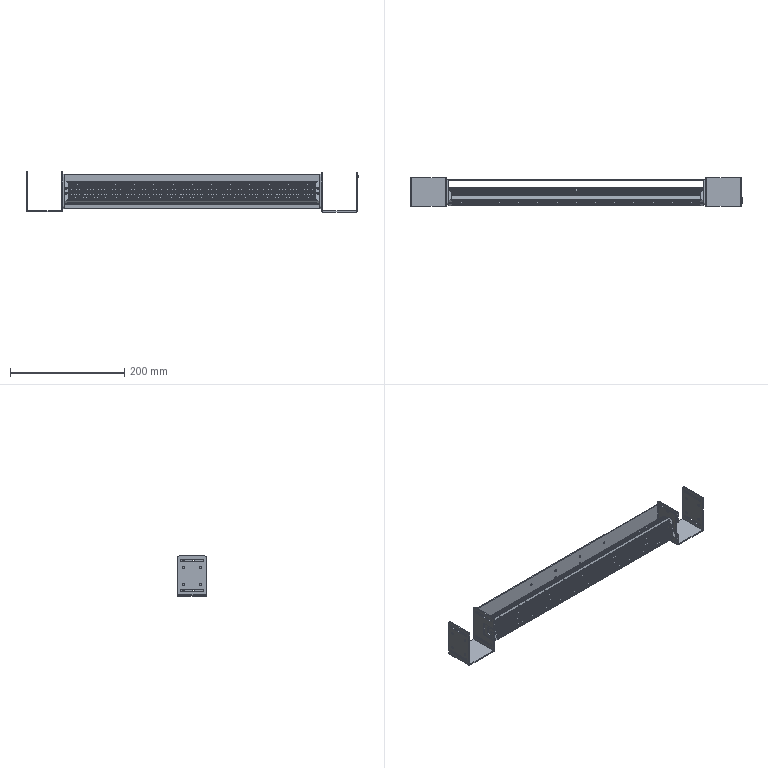Part | SolidWorks | 24 solids | 3125 faces | volume 224548 mm3 | spline 1080 | cylinder 908 | plane 887 | cone 250 | commonest cylinder face diameters 2 x434 1.9 x216 0.2 x90 3.3 x52 0.6 x24 4.5 x22